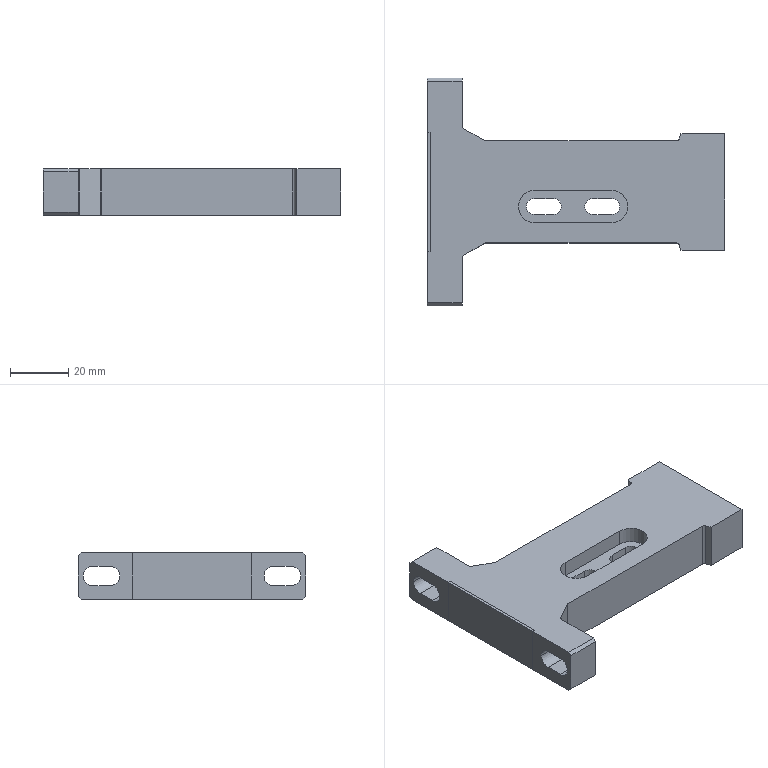NC program | NX | posted with a generic post | part box 102 x 78 x 16 mm
Lines 2750 to 3711 of 11044:
(ZLEVEL_PROFILE_COPY_COPY_1_COPY , TOOL : D4)
N5474 T04 M6
N5476 G54
N5478 G17 G0 G90 X-36. Y25.848 B0. C0. S9500 M3
N5480 G43 Z30. H4
N5482 Z-0.4
N5484 G94 G1 X-36.8 Y25.386 F1400.
N5486 G3 X-37. Y25.039 R0.4
N5488 G1 Y23.155
N5490 X-35.367 Y22.212
N5492 G3 X-34.967 Y22.212 R0.4
N5494 G1 X-34.167 Y22.674
N5496 G0 X-36. Y25.848 Z-0.8
N5498 G1 X-36.8 Y25.386
N5500 G3 X-37. Y25.039 R0.4
N5502 G1 Y23.155
N5504 X-35.367 Y22.212
N5506 G3 X-34.967 Y22.212 R0.4
N5508 G1 X-34.167 Y22.674
N5510 G0 X-36. Y25.848 Z-1.2
N5512 G1 X-36.8 Y25.386
N5514 G3 X-37. Y25.039 R0.4
N5516 G1 Y23.155
N5518 X-35.367 Y22.212
N5520 G3 X-34.967 Y22.212 R0.4
N5522 G1 X-34.167 Y22.674
N5524 G0 X-36. Y25.848 Z-1.6
N5526 G1 X-36.8 Y25.386
N5528 G3 X-37. Y25.039 R0.4
N5530 G1 Y23.155
N5532 X-35.367 Y22.212
N5534 G3 X-34.967 Y22.212 R0.4
N5536 G1 X-34.167 Y22.674
N5538 G0 X-36. Y25.848 Z-2.
N5540 G1 X-36.8 Y25.386
N5542 G3 X-37. Y25.039 R0.4
N5544 G1 Y23.155
N5546 X-35.367 Y22.212
N5548 G3 X-34.967 Y22.212 R0.4
N5550 G1 X-34.167 Y22.674
N5552 G0 X-36. Y25.848 Z-2.4
N5554 G1 X-36.8 Y25.386
N5556 G3 X-37. Y25.039 R0.4
N5558 G1 Y23.155
N5560 X-35.367 Y22.212
N5562 G3 X-34.967 Y22.212 R0.4
N5564 G1 X-34.167 Y22.674
N5566 G0 X-36. Y25.848 Z-2.8
N5568 G1 X-36.8 Y25.386
N5570 G3 X-37. Y25.039 R0.4
N5572 G1 Y23.155
N5574 X-35.367 Y22.212
N5576 G3 X-34.967 Y22.212 R0.4
N5578 G1 X-34.167 Y22.674
N5580 G0 X-36. Y25.848 Z-3.2
N5582 G1 X-36.8 Y25.386
N5584 G3 X-37. Y25.039 R0.4
N5586 G1 Y23.155
N5588 X-35.367 Y22.212
N5590 G3 X-34.967 Y22.212 R0.4
N5592 G1 X-34.167 Y22.674
N5594 G0 X-36. Y25.848 Z-3.6
N5596 G1 X-36.8 Y25.386
N5598 G3 X-37. Y25.039 R0.4
N5600 G1 Y23.155
N5602 X-35.367 Y22.212
N5604 G3 X-34.967 Y22.212 R0.4
N5606 G1 X-34.167 Y22.674
N5608 G0 X-36. Y25.848 Z-4.
N5610 G1 X-36.8 Y25.386
N5612 G3 X-37. Y25.039 R0.4
N5614 G1 Y23.155
N5616 X-35.367 Y22.212
N5618 G3 X-34.967 Y22.212 R0.4
N5620 G1 X-34.167 Y22.674
N5622 G0 X-36. Y25.848 Z-4.4
N5624 G1 X-36.8 Y25.386
N5626 G3 X-37. Y25.039 R0.4
N5628 G1 Y23.155
N5630 X-35.367 Y22.212
N5632 G3 X-34.967 Y22.212 R0.4
N5634 G1 X-34.167 Y22.674
N5636 G0 X-36. Y25.848 Z-4.8
N5638 G1 X-36.8 Y25.386
N5640 G3 X-37. Y25.039 R0.4
N5642 G1 Y23.155
N5644 X-35.367 Y22.212
N5646 G3 X-34.967 Y22.212 R0.4
N5648 G1 X-34.167 Y22.674
N5650 G0 X-36. Y25.848 Z-5.2
N5652 G1 X-36.8 Y25.386
N5654 G3 X-37. Y25.039 R0.4
N5656 G1 Y23.155
N5658 X-35.367 Y22.212
N5660 G3 X-34.967 Y22.212 R0.4
N5662 G1 X-34.167 Y22.674
N5664 G0 X-36. Y25.848 Z-5.6
N5666 G1 X-36.8 Y25.386
N5668 G3 X-37. Y25.039 R0.4
N5670 G1 Y23.155
N5672 X-35.367 Y22.212
N5674 G3 X-34.967 Y22.212 R0.4
N5676 G1 X-34.167 Y22.674
N5678 G0 X-36. Y25.848 Z-6.
N5680 G1 X-36.8 Y25.386
N5682 G3 X-37. Y25.039 R0.4
N5684 G1 Y23.155
N5686 X-35.367 Y22.212
N5688 G3 X-34.967 Y22.212 R0.4
N5690 G1 X-34.167 Y22.674
N5692 G0 X-36. Y25.848 Z-6.4
N5694 G1 X-36.8 Y25.386
N5696 G3 X-37. Y25.039 R0.4
N5698 G1 Y23.155
N5700 X-35.367 Y22.212
N5702 G3 X-34.967 Y22.212 R0.4
N5704 G1 X-34.167 Y22.674
N5706 G0 X-36. Y25.848 Z-6.8
N5708 G1 X-36.8 Y25.386
N5710 G3 X-37. Y25.039 R0.4
N5712 G1 Y23.155
N5714 X-35.367 Y22.212
N5716 G3 X-34.967 Y22.212 R0.4
N5718 G1 X-34.167 Y22.674
N5720 G0 X-36. Y25.848 Z-7.2
N5722 G1 X-36.8 Y25.386
N5724 G3 X-37. Y25.039 R0.4
N5726 G1 Y23.155
N5728 X-35.367 Y22.212
N5730 G3 X-34.967 Y22.212 R0.4
N5732 G1 X-34.167 Y22.674
N5734 G0 X-36. Y25.848 Z-7.6
N5736 G1 X-36.8 Y25.386
N5738 G3 X-37. Y25.039 R0.4
N5740 G1 Y23.155
N5742 X-35.367 Y22.212
N5744 G3 X-34.967 Y22.212 R0.4
N5746 G1 X-34.167 Y22.674
N5748 G0 X-36. Y25.848 Z-8.
N5750 G1 X-36.8 Y25.386
N5752 G3 X-37. Y25.039 R0.4
N5754 G1 Y23.155
N5756 X-35.367 Y22.212
N5758 G3 X-34.967 Y22.212 R0.4
N5760 G1 X-34.167 Y22.674
N5762 G0 X-36. Y25.848 Z-8.4
N5764 G1 X-36.8 Y25.386
N5766 G3 X-37. Y25.039 R0.4
N5768 G1 Y23.155
N5770 X-35.367 Y22.212
N5772 G3 X-34.967 Y22.212 R0.4
N5774 G1 X-34.167 Y22.674
N5776 G0 X-36. Y25.848 Z-8.8
N5778 G1 X-36.8 Y25.386
N5780 G3 X-37. Y25.039 R0.4
N5782 G1 Y23.155
N5784 X-35.367 Y22.212
N5786 G3 X-34.967 Y22.212 R0.4
N5788 G1 X-34.167 Y22.674
N5790 G0 X-36. Y25.848 Z-9.2
N5792 G1 X-36.8 Y25.386
N5794 G3 X-37. Y25.039 R0.4
N5796 G1 Y23.155
N5798 X-35.367 Y22.212
N5800 G3 X-34.967 Y22.212 R0.4
N5802 G1 X-34.167 Y22.674
N5804 G0 X-36. Y25.848 Z-9.6
N5806 G1 X-36.8 Y25.386
N5808 G3 X-37. Y25.039 R0.4
N5810 G1 Y23.155
N5812 X-35.367 Y22.212
N5814 G3 X-34.967 Y22.212 R0.4
N5816 G1 X-34.167 Y22.674
N5818 G0 X-36. Y25.848 Z-10.
N5820 G1 X-36.8 Y25.386
N5822 G3 X-37. Y25.039 R0.4
N5824 G1 Y23.155
N5826 X-35.367 Y22.212
N5828 G3 X-34.967 Y22.212 R0.4
N5830 G1 X-34.167 Y22.674
N5832 G0 X-36. Y25.848 Z-10.4
N5834 G1 X-36.8 Y25.386
N5836 G3 X-37. Y25.039 R0.4
N5838 G1 Y23.155
N5840 X-35.367 Y22.212
N5842 G3 X-34.967 Y22.212 R0.4
N5844 G1 X-34.167 Y22.674
N5846 G0 X-36. Y25.848 Z-10.8
N5848 G1 X-36.8 Y25.386
N5850 G3 X-37. Y25.039 R0.4
N5852 G1 Y23.155
N5854 X-35.367 Y22.212
N5856 G3 X-34.967 Y22.212 R0.4
N5858 G1 X-34.167 Y22.674
N5860 G0 X-36. Y25.848 Z-11.2
N5862 G1 X-36.8 Y25.386
N5864 G3 X-37. Y25.039 R0.4
N5866 G1 Y23.155
N5868 X-35.367 Y22.212
N5870 G3 X-34.967 Y22.212 R0.4
N5872 G1 X-34.167 Y22.674
N5874 G0 X-36. Y25.848 Z-11.6
N5876 G1 X-36.8 Y25.386
N5878 G3 X-37. Y25.039 R0.4
N5880 G1 Y23.155
N5882 X-35.367 Y22.212
N5884 G3 X-34.967 Y22.212 R0.4
N5886 G1 X-34.167 Y22.674
N5888 G0 X-36. Y25.848 Z-12.
N5890 G1 X-36.8 Y25.386
N5892 G3 X-37. Y25.039 R0.4
N5894 G1 Y23.155
N5896 X-35.367 Y22.212
N5898 G3 X-34.967 Y22.212 R0.4
N5900 G1 X-34.167 Y22.674
N5902 G0 X-36. Y25.848 Z-12.4
N5904 G1 X-36.8 Y25.386
N5906 G3 X-37. Y25.039 R0.4
N5908 G1 Y23.155
N5910 X-35.367 Y22.212
N5912 G3 X-34.967 Y22.212 R0.4
N5914 G1 X-34.167 Y22.674
N5916 G0 X-36. Y25.848 Z-12.8
N5918 G1 X-36.8 Y25.386
N5920 G3 X-37. Y25.039 R0.4
N5922 G1 Y23.155
N5924 X-35.367 Y22.212
N5926 G3 X-34.967 Y22.212 R0.4
N5928 G1 X-34.167 Y22.674
N5930 G0 X-36. Y25.848 Z-13.2
N5932 G1 X-36.8 Y25.386
N5934 G3 X-37. Y25.039 R0.4
N5936 G1 Y23.155
N5938 X-35.367 Y22.212
N5940 G3 X-34.967 Y22.212 R0.4
N5942 G1 X-34.167 Y22.674
N5944 G0 X-36. Y25.848 Z-13.6
N5946 G1 X-36.8 Y25.386
N5948 G3 X-37. Y25.039 R0.4
N5950 G1 Y23.155
N5952 X-35.367 Y22.212
N5954 G3 X-34.967 Y22.212 R0.4
N5956 G1 X-34.167 Y22.674
N5958 G0 X-36. Y25.848 Z-14.
N5960 G1 X-36.8 Y25.386
N5962 G3 X-37. Y25.039 R0.4
N5964 G1 Y23.155
N5966 X-35.367 Y22.212
N5968 G3 X-34.967 Y22.212 R0.4
N5970 G1 X-34.167 Y22.674
N5972 G0 X-36. Y25.848 Z-14.4
N5974 G1 X-36.8 Y25.386
N5976 G3 X-37. Y25.039 R0.4
N5978 G1 Y23.155
N5980 X-35.367 Y22.212
N5982 G3 X-34.967 Y22.212 R0.4
N5984 G1 X-34.167 Y22.674
N5986 G0 X-36. Y25.848 Z-14.8
N5988 G1 X-36.8 Y25.386
N5990 G3 X-37. Y25.039 R0.4
N5992 G1 Y23.155
N5994 X-35.367 Y22.212
N5996 G3 X-34.967 Y22.212 R0.4
N5998 G1 X-34.167 Y22.674
N6000 G0 X-36. Y25.848 Z-15.2
N6002 G1 X-36.8 Y25.386
N6004 G3 X-37. Y25.039 R0.4
N6006 G1 Y23.155
N6008 X-35.367 Y22.212
N6010 G3 X-34.967 Y22.212 R0.4
N6012 G1 X-34.167 Y22.674
N6014 G0 X-36. Y25.848 Z-15.6
N6016 G1 X-36.8 Y25.386
N6018 G3 X-37. Y25.039 R0.4
N6020 G1 Y23.155
N6022 X-35.367 Y22.212
N6024 G3 X-34.967 Y22.212 R0.4
N6026 G1 X-34.167 Y22.674
N6028 G0 X-36. Y25.848 Z-16.
N6030 G1 X-36.8 Y25.386
N6032 G3 X-37. Y25.039 R0.4
N6034 G1 Y23.155
N6036 X-35.367 Y22.212
N6038 G3 X-34.967 Y22.212 R0.4
N6040 G1 X-34.167 Y22.674
N6042 G0 Z30.
N6044 X-31.699 Y21.249
N6046 Z-0.4
N6048 G1 Y20.325
N6050 G3 X-31.499 Y19.978 R0.4
N6052 G1 X-30.67 Y19.5
N6054 X-29.713
N6056 G3 X-29.367 Y19.7 R0.4
N6058 G1 X-28.905 Y20.5
N6060 G0 X-31.699 Y21.249 Z-0.8
N6062 G1 Y20.325
N6064 G3 X-31.499 Y19.978 R0.4
N6066 G1 X-30.67 Y19.5
N6068 X-29.713
N6070 G3 X-29.367 Y19.7 R0.4
N6072 G1 X-28.905 Y20.5
N6074 G0 X-31.699 Y21.249 Z-1.2
N6076 G1 Y20.325
N6078 G3 X-31.499 Y19.978 R0.4
N6080 G1 X-30.67 Y19.5
N6082 X-29.713
N6084 G3 X-29.367 Y19.7 R0.4
N6086 G1 X-28.905 Y20.5
N6088 G0 X-31.699 Y21.249 Z-1.6
N6090 G1 Y20.325
N6092 G3 X-31.499 Y19.978 R0.4
N6094 G1 X-30.67 Y19.5
N6096 X-29.713
N6098 G3 X-29.367 Y19.7 R0.4
N6100 G1 X-28.905 Y20.5
N6102 G0 X-31.699 Y21.249 Z-2.
N6104 G1 Y20.325
N6106 G3 X-31.499 Y19.978 R0.4
N6108 G1 X-30.67 Y19.5
N6110 X-29.713
N6112 G3 X-29.367 Y19.7 R0.4
N6114 G1 X-28.905 Y20.5
N6116 G0 X-31.699 Y21.249 Z-2.4
N6118 G1 Y20.325
N6120 G3 X-31.499 Y19.978 R0.4
N6122 G1 X-30.67 Y19.5
N6124 X-29.713
N6126 G3 X-29.367 Y19.7 R0.4
N6128 G1 X-28.905 Y20.5
N6130 G0 X-31.699 Y21.249 Z-2.8
N6132 G1 Y20.325
N6134 G3 X-31.499 Y19.978 R0.4
N6136 G1 X-30.67 Y19.5
N6138 X-29.713
N6140 G3 X-29.367 Y19.7 R0.4
N6142 G1 X-28.905 Y20.5
N6144 G0 X-31.699 Y21.249 Z-3.2
N6146 G1 Y20.325
N6148 G3 X-31.499 Y19.978 R0.4
N6150 G1 X-30.67 Y19.5
N6152 X-29.713
N6154 G3 X-29.367 Y19.7 R0.4
N6156 G1 X-28.905 Y20.5
N6158 G0 X-31.699 Y21.249 Z-3.6
N6160 G1 Y20.325
N6162 G3 X-31.499 Y19.978 R0.4
N6164 G1 X-30.67 Y19.5
N6166 X-29.713
N6168 G3 X-29.367 Y19.7 R0.4
N6170 G1 X-28.905 Y20.5
N6172 G0 X-31.699 Y21.249 Z-4.
N6174 G1 Y20.325
N6176 G3 X-31.499 Y19.978 R0.4
N6178 G1 X-30.67 Y19.5
N6180 X-29.713
N6182 G3 X-29.367 Y19.7 R0.4
N6184 G1 X-28.905 Y20.5
N6186 G0 X-31.699 Y21.249 Z-4.4
N6188 G1 Y20.325
N6190 G3 X-31.499 Y19.978 R0.4
N6192 G1 X-30.67 Y19.5
N6194 X-29.713
N6196 G3 X-29.367 Y19.7 R0.4
N6198 G1 X-28.905 Y20.5
N6200 G0 X-31.699 Y21.249 Z-4.8
N6202 G1 Y20.325
N6204 G3 X-31.499 Y19.978 R0.4
N6206 G1 X-30.67 Y19.5
N6208 X-29.713
N6210 G3 X-29.367 Y19.7 R0.4
N6212 G1 X-28.905 Y20.5
N6214 G0 X-31.699 Y21.249 Z-5.2
N6216 G1 Y20.325
N6218 G3 X-31.499 Y19.978 R0.4
N6220 G1 X-30.67 Y19.5
N6222 X-29.713
N6224 G3 X-29.367 Y19.7 R0.4
N6226 G1 X-28.905 Y20.5
N6228 G0 X-31.699 Y21.249 Z-5.6
N6230 G1 Y20.325
N6232 G3 X-31.499 Y19.978 R0.4
N6234 G1 X-30.67 Y19.5
N6236 X-29.713
N6238 G3 X-29.367 Y19.7 R0.4
N6240 G1 X-28.905 Y20.5
N6242 G0 X-31.699 Y21.249 Z-6.
N6244 G1 Y20.325
N6246 G3 X-31.499 Y19.978 R0.4
N6248 G1 X-30.67 Y19.5
N6250 X-29.713
N6252 G3 X-29.367 Y19.7 R0.4
N6254 G1 X-28.905 Y20.5
N6256 G0 X-31.699 Y21.249 Z-6.4
N6258 G1 Y20.325
N6260 G3 X-31.499 Y19.978 R0.4
N6262 G1 X-30.67 Y19.5
N6264 X-29.713
N6266 G3 X-29.367 Y19.7 R0.4
N6268 G1 X-28.905 Y20.5
N6270 G0 X-31.699 Y21.249 Z-6.8
N6272 G1 Y20.325
N6274 G3 X-31.499 Y19.978 R0.4
N6276 G1 X-30.67 Y19.5
N6278 X-29.713
N6280 G3 X-29.367 Y19.7 R0.4
N6282 G1 X-28.905 Y20.5
N6284 G0 X-31.699 Y21.249 Z-7.2
N6286 G1 Y20.325
N6288 G3 X-31.499 Y19.978 R0.4
N6290 G1 X-30.67 Y19.5
N6292 X-29.713
N6294 G3 X-29.367 Y19.7 R0.4
N6296 G1 X-28.905 Y20.5
N6298 G0 X-31.699 Y21.249 Z-7.6
N6300 G1 Y20.325
N6302 G3 X-31.499 Y19.978 R0.4
N6304 G1 X-30.67 Y19.5
N6306 X-29.713
N6308 G3 X-29.367 Y19.7 R0.4
N6310 G1 X-28.905 Y20.5
N6312 G0 X-31.699 Y21.249 Z-8.
N6314 G1 Y20.325
N6316 G3 X-31.499 Y19.978 R0.4
N6318 G1 X-30.67 Y19.5
N6320 X-29.713
N6322 G3 X-29.367 Y19.7 R0.4
N6324 G1 X-28.905 Y20.5
N6326 G0 X-31.699 Y21.249 Z-8.4
N6328 G1 Y20.325
N6330 G3 X-31.499 Y19.978 R0.4
N6332 G1 X-30.67 Y19.5
N6334 X-29.713
N6336 G3 X-29.367 Y19.7 R0.4
N6338 G1 X-28.905 Y20.5
N6340 G0 X-31.699 Y21.249 Z-8.8
N6342 G1 Y20.325
N6344 G3 X-31.499 Y19.978 R0.4
N6346 G1 X-30.67 Y19.5
N6348 X-29.713
N6350 G3 X-29.367 Y19.7 R0.4
N6352 G1 X-28.905 Y20.5
N6354 G0 X-31.699 Y21.249 Z-9.2
N6356 G1 Y20.325
N6358 G3 X-31.499 Y19.978 R0.4
N6360 G1 X-30.67 Y19.5
N6362 X-29.713
N6364 G3 X-29.367 Y19.7 R0.4
N6366 G1 X-28.905 Y20.5
N6368 G0 X-31.699 Y21.249 Z-9.6
N6370 G1 Y20.325
N6372 G3 X-31.499 Y19.978 R0.4
N6374 G1 X-30.67 Y19.5
N6376 X-29.713
N6378 G3 X-29.367 Y19.7 R0.4
N6380 G1 X-28.905 Y20.5
N6382 G0 X-31.699 Y21.249 Z-10.
N6384 G1 Y20.325
N6386 G3 X-31.499 Y19.978 R0.4
N6388 G1 X-30.67 Y19.5
N6390 X-29.713
N6392 G3 X-29.367 Y19.7 R0.4
N6394 G1 X-28.905 Y20.5
N6396 G0 X-31.699 Y21.249 Z-10.4
N6398 G1 Y20.325
N6400 G3 X-31.499 Y19.978 R0.4
N6402 G1 X-30.67 Y19.5
N6404 X-29.713
N6406 G3 X-29.367 Y19.7 R0.4
N6408 G1 X-28.905 Y20.5
N6410 G0 X-31.699 Y21.249 Z-10.8
N6412 G1 Y20.325
N6414 G3 X-31.499 Y19.978 R0.4
N6416 G1 X-30.67 Y19.5
N6418 X-29.713
N6420 G3 X-29.367 Y19.7 R0.4
N6422 G1 X-28.905 Y20.5
N6424 G0 X-31.699 Y21.249 Z-11.2
N6426 G1 Y20.325
N6428 G3 X-31.499 Y19.978 R0.4
N6430 G1 X-30.67 Y19.5
N6432 X-29.713
N6434 G3 X-29.367 Y19.7 R0.4
N6436 G1 X-28.905 Y20.5
N6438 G0 X-31.699 Y21.249 Z-11.6
N6440 G1 Y20.325
N6442 G3 X-31.499 Y19.978 R0.4
N6444 G1 X-30.67 Y19.5
N6446 X-29.713
N6448 G3 X-29.367 Y19.7 R0.4
N6450 G1 X-28.905 Y20.5
N6452 G0 X-31.699 Y21.249 Z-12.
N6454 G1 Y20.325
N6456 G3 X-31.499 Y19.978 R0.4
N6458 G1 X-30.67 Y19.5
N6460 X-29.713
N6462 G3 X-29.367 Y19.7 R0.4
N6464 G1 X-28.905 Y20.5
N6466 G0 X-31.699 Y21.249 Z-12.4
N6468 G1 Y20.325
N6470 G3 X-31.499 Y19.978 R0.4
N6472 G1 X-30.67 Y19.5
N6474 X-29.713
N6476 G3 X-29.367 Y19.7 R0.4
N6478 G1 X-28.905 Y20.5
N6480 G0 X-31.699 Y21.249 Z-12.8
N6482 G1 Y20.325
N6484 G3 X-31.499 Y19.978 R0.4
N6486 G1 X-30.67 Y19.5
N6488 X-29.713
N6490 G3 X-29.367 Y19.7 R0.4
N6492 G1 X-28.905 Y20.5
N6494 G0 X-31.699 Y21.249 Z-13.2
N6496 G1 Y20.325
N6498 G3 X-31.499 Y19.978 R0.4
N6500 G1 X-30.67 Y19.5
N6502 X-29.713
N6504 G3 X-29.367 Y19.7 R0.4
N6506 G1 X-28.905 Y20.5
N6508 G0 X-31.699 Y21.249 Z-13.6
N6510 G1 Y20.325
N6512 G3 X-31.499 Y19.978 R0.4
N6514 G1 X-30.67 Y19.5
N6516 X-29.713
N6518 G3 X-29.367 Y19.7 R0.4
N6520 G1 X-28.905 Y20.5
N6522 G0 X-31.699 Y21.249 Z-14.
N6524 G1 Y20.325
N6526 G3 X-31.499 Y19.978 R0.4
N6528 G1 X-30.67 Y19.5
N6530 X-29.713
N6532 G3 X-29.367 Y19.7 R0.4
N6534 G1 X-28.905 Y20.5
N6536 G0 X-31.699 Y21.249 Z-14.4
N6538 G1 Y20.325
N6540 G3 X-31.499 Y19.978 R0.4
N6542 G1 X-30.67 Y19.5
N6544 X-29.713
N6546 G3 X-29.367 Y19.7 R0.4
N6548 G1 X-28.905 Y20.5
N6550 G0 X-31.699 Y21.249 Z-14.8
N6552 G1 Y20.325
N6554 G3 X-31.499 Y19.978 R0.4
N6556 G1 X-30.67 Y19.5
N6558 X-29.713
N6560 G3 X-29.367 Y19.7 R0.4
N6562 G1 X-28.905 Y20.5
N6564 G0 X-31.699 Y21.249 Z-15.2
N6566 G1 Y20.325
N6568 G3 X-31.499 Y19.978 R0.4
N6570 G1 X-30.67 Y19.5
N6572 X-29.713
N6574 G3 X-29.367 Y19.7 R0.4
N6576 G1 X-28.905 Y20.5
N6578 G0 X-31.699 Y21.249 Z-15.6
N6580 G1 Y20.325
N6582 G3 X-31.499 Y19.978 R0.4
N6584 G1 X-30.67 Y19.5
N6586 X-29.713
N6588 G3 X-29.367 Y19.7 R0.4
N6590 G1 X-28.905 Y20.5
N6592 G0 X-31.699 Y21.249 Z-16.
N6594 G1 Y20.325
N6596 G3 X-31.499 Y19.978 R0.4
N6598 G1 X-30.67 Y19.5
N6600 X-29.713
N6602 G3 X-29.367 Y19.7 R0.4
N6604 G1 X-28.905 Y20.5
N6606 G0 Z30.
N6608 X30.709
N6610 Z-0.4
N6612 G1 X31.17 Y19.7
N6614 G3 X31.517 Y19.5 R0.4
N6616 G1 X33.69
N6618 X34.121 Y20.684
N6620 G2 X34.426 Y21.233 R2.
N6622 G3 X34.482 Y21.629 R0.4
N6624 G1 X34.178 Y22.383
N6626 G0 X30.709 Y20.5 Z-0.8
N6628 G1 X31.17 Y19.7
N6630 G3 X31.517 Y19.5 R0.4
N6632 G1 X33.69
N6634 X34.121 Y20.684
N6636 G2 X34.426 Y21.233 R2.
N6638 G3 X34.482 Y21.629 R0.4
N6640 G1 X34.178 Y22.383
N6642 G0 X30.709 Y20.5 Z-1.2
N6644 G1 X31.17 Y19.7
N6646 G3 X31.517 Y19.5 R0.4
N6648 G1 X33.69
N6650 X34.121 Y20.684
N6652 G2 X34.426 Y21.233 R2.
N6654 G3 X34.482 Y21.629 R0.4
N6656 G1 X34.178 Y22.383
N6658 G0 X30.709 Y20.5 Z-1.6
N6660 G1 X31.17 Y19.7
N6662 G3 X31.517 Y19.5 R0.4
N6664 G1 X33.69
N6666 X34.121 Y20.684
N6668 G2 X34.426 Y21.233 R2.
N6670 G3 X34.482 Y21.629 R0.4
N6672 G1 X34.178 Y22.383
N6674 G0 X30.709 Y20.5 Z-2.
N6676 G1 X31.17 Y19.7
N6678 G3 X31.517 Y19.5 R0.4
N6680 G1 X33.69
N6682 X34.121 Y20.684
N6684 G2 X34.426 Y21.233 R2.
N6686 G3 X34.482 Y21.629 R0.4
N6688 G1 X34.178 Y22.383
N6690 G0 X30.709 Y20.5 Z-2.4
N6692 G1 X31.17 Y19.7
N6694 G3 X31.517 Y19.5 R0.4
N6696 G1 X33.69
N6698 X34.121 Y20.684
N6700 G2 X34.426 Y21.233 R2.
N6702 G3 X34.482 Y21.629 R0.4
N6704 G1 X34.178 Y22.383
N6706 G0 X30.709 Y20.5 Z-2.8
N6708 G1 X31.17 Y19.7
N6710 G3 X31.517 Y19.5 R0.4
N6712 G1 X33.69
N6714 X34.121 Y20.684
N6716 G2 X34.426 Y21.233 R2.
N6718 G3 X34.482 Y21.629 R0.4
N6720 G1 X34.178 Y22.383
N6722 G0 X30.709 Y20.5 Z-3.2
N6724 G1 X31.17 Y19.7
N6726 G3 X31.517 Y19.5 R0.4
N6728 G1 X33.69
N6730 X34.121 Y20.684
N6732 G2 X34.426 Y21.233 R2.
N6734 G3 X34.482 Y21.629 R0.4
N6736 G1 X34.178 Y22.383
N6738 G0 X30.709 Y20.5 Z-3.6
N6740 G1 X31.17 Y19.7
N6742 G3 X31.517 Y19.5 R0.4
N6744 G1 X33.69
N6746 X34.121 Y20.684
N6748 G2 X34.426 Y21.233 R2.
N6750 G3 X34.482 Y21.629 R0.4
N6752 G1 X34.178 Y22.383
N6754 G0 X30.709 Y20.5 Z-4.
N6756 G1 X31.17 Y19.7
N6758 G3 X31.517 Y19.5 R0.4
N6760 G1 X33.69
N6762 X34.121 Y20.684
N6764 G2 X34.426 Y21.233 R2.
N6766 G3 X34.482 Y21.629 R0.4
N6768 G1 X34.178 Y22.383
N6770 G0 X30.709 Y20.5 Z-4.4
N6772 G1 X31.17 Y19.7
N6774 G3 X31.517 Y19.5 R0.4
N6776 G1 X33.69
N6778 X34.121 Y20.684
N6780 G2 X34.426 Y21.233 R2.
N6782 G3 X34.482 Y21.629 R0.4
N6784 G1 X34.178 Y22.383
N6786 G0 X30.709 Y20.5 Z-4.8
N6788 G1 X31.17 Y19.7
N6790 G3 X31.517 Y19.5 R0.4
N6792 G1 X33.69
N6794 X34.121 Y20.684
N6796 G2 X34.426 Y21.233 R2.
N6798 G3 X34.482 Y21.629 R0.4
N6800 G1 X34.178 Y22.383
N6802 G0 X30.709 Y20.5 Z-5.2
N6804 G1 X31.17 Y19.7
N6806 G3 X31.517 Y19.5 R0.4
N6808 G1 X33.69
N6810 X34.121 Y20.684
N6812 G2 X34.426 Y21.233 R2.
N6814 G3 X34.482 Y21.629 R0.4
N6816 G1 X34.178 Y22.383
N6818 G0 X30.709 Y20.5 Z-5.6
N6820 G1 X31.17 Y19.7
N6822 G3 X31.517 Y19.5 R0.4
N6824 G1 X33.69
N6826 X34.121 Y20.684
N6828 G2 X34.426 Y21.233 R2.
N6830 G3 X34.482 Y21.629 R0.4
N6832 G1 X34.178 Y22.383
N6834 G0 X30.709 Y20.5 Z-6.
N6836 G1 X31.17 Y19.7
N6838 G3 X31.517 Y19.5 R0.4
N6840 G1 X33.69
N6842 X34.121 Y20.684
N6844 G2 X34.426 Y21.233 R2.
N6846 G3 X34.482 Y21.629 R0.4
N6848 G1 X34.178 Y22.383
N6850 G0 X30.709 Y20.5 Z-6.4
N6852 G1 X31.17 Y19.7
N6854 G3 X31.517 Y19.5 R0.4
N6856 G1 X33.69
N6858 X34.121 Y20.684
N6860 G2 X34.426 Y21.233 R2.
N6862 G3 X34.482 Y21.629 R0.4
N6864 G1 X34.178 Y22.383
N6866 G0 X30.709 Y20.5 Z-6.8
N6868 G1 X31.17 Y19.7
N6870 G3 X31.517 Y19.5 R0.4
N6872 G1 X33.69
N6874 X34.121 Y20.684
N6876 G2 X34.426 Y21.233 R2.
N6878 G3 X34.482 Y21.629 R0.4
N6880 G1 X34.178 Y22.383
N6882 G0 X30.709 Y20.5 Z-7.2
N6884 G1 X31.17 Y19.7
N6886 G3 X31.517 Y19.5 R0.4
N6888 G1 X33.69
N6890 X34.121 Y20.684
N6892 G2 X34.426 Y21.233 R2.
N6894 G3 X34.482 Y21.629 R0.4
N6896 G1 X34.178 Y22.383
N6898 G0 X30.709 Y20.5 Z-7.6
N6900 G1 X31.17 Y19.7
N6902 G3 X31.517 Y19.5 R0.4
N6904 G1 X33.69
N6906 X34.121 Y20.684
N6908 G2 X34.426 Y21.233 R2.
N6910 G3 X34.482 Y21.629 R0.4
N6912 G1 X34.178 Y22.383
N6914 G0 X30.709 Y20.5 Z-8.
N6916 G1 X31.17 Y19.7
N6918 G3 X31.517 Y19.5 R0.4
N6920 G1 X33.69
N6922 X34.121 Y20.684
N6924 G2 X34.426 Y21.233 R2.
N6926 G3 X34.482 Y21.629 R0.4
N6928 G1 X34.178 Y22.383
N6930 G0 X30.709 Y20.5 Z-8.4
N6932 G1 X31.17 Y19.7
N6934 G3 X31.517 Y19.5 R0.4
N6936 G1 X33.69
N6938 X34.121 Y20.684
N6940 G2 X34.426 Y21.233 R2.
N6942 G3 X34.482 Y21.629 R0.4
N6944 G1 X34.178 Y22.383
N6946 G0 X30.709 Y20.5 Z-8.8
N6948 G1 X31.17 Y19.7
N6950 G3 X31.517 Y19.5 R0.4
N6952 G1 X33.69
N6954 X34.121 Y20.684
N6956 G2 X34.426 Y21.233 R2.
N6958 G3 X34.482 Y21.629 R0.4
N6960 G1 X34.178 Y22.383
N6962 G0 X30.709 Y20.5 Z-9.2
N6964 G1 X31.17 Y19.7
N6966 G3 X31.517 Y19.5 R0.4
N6968 G1 X33.69
N6970 X34.121 Y20.684
N6972 G2 X34.426 Y21.233 R2.
N6974 G3 X34.482 Y21.629 R0.4
N6976 G1 X34.178 Y22.383
N6978 G0 X30.709 Y20.5 Z-9.6
N6980 G1 X31.17 Y19.7
N6982 G3 X31.517 Y19.5 R0.4
N6984 G1 X33.69
N6986 X34.121 Y20.684
N6988 G2 X34.426 Y21.233 R2.
N6990 G3 X34.482 Y21.629 R0.4
N6992 G1 X34.178 Y22.383
N6994 G0 X30.709 Y20.5 Z-10.
N6996 G1 X31.17 Y19.7
N6998 G3 X31.517 Y19.5 R0.4
N7000 G1 X33.69
N7002 X34.121 Y20.684
N7004 G2 X34.426 Y21.233 R2.
N7006 G3 X34.482 Y21.629 R0.4
N7008 G1 X34.178 Y22.383
N7010 G0 X30.709 Y20.5 Z-10.4
N7012 G1 X31.17 Y19.7
N7014 G3 X31.517 Y19.5 R0.4
N7016 G1 X33.69
N7018 X34.121 Y20.684
N7020 G2 X34.426 Y21.233 R2.
N7022 G3 X34.482 Y21.629 R0.4
N7024 G1 X34.178 Y22.383
N7026 G0 X30.709 Y20.5 Z-10.8
N7028 G1 X31.17 Y19.7
N7030 G3 X31.517 Y19.5 R0.4
N7032 G1 X33.69
N7034 X34.121 Y20.684
N7036 G2 X34.426 Y21.233 R2.
N7038 G3 X34.482 Y21.629 R0.4
N7040 G1 X34.178 Y22.383
N7042 G0 X30.709 Y20.5 Z-11.2
N7044 G1 X31.17 Y19.7
N7046 G3 X31.517 Y19.5 R0.4
N7048 G1 X33.69
N7050 X34.121 Y20.684
N7052 G2 X34.426 Y21.233 R2.
N7054 G3 X34.482 Y21.629 R0.4
N7056 G1 X34.178 Y22.383
N7058 G0 X30.709 Y20.5 Z-11.6
N7060 G1 X31.17 Y19.7
N7062 G3 X31.517 Y19.5 R0.4
N7064 G1 X33.69
N7066 X34.121 Y20.684
N7068 G2 X34.426 Y21.233 R2.
N7070 G3 X34.482 Y21.629 R0.4
N7072 G1 X34.178 Y22.383
N7074 G0 X30.709 Y20.5 Z-12.
N7076 G1 X31.17 Y19.7
N7078 G3 X31.517 Y19.5 R0.4
N7080 G1 X33.69
N7082 X34.121 Y20.684
N7084 G2 X34.426 Y21.233 R2.
N7086 G3 X34.482 Y21.629 R0.4
N7088 G1 X34.178 Y22.383
N7090 G0 X30.709 Y20.5 Z-12.4
N7092 G1 X31.17 Y19.7
N7094 G3 X31.517 Y19.5 R0.4
N7096 G1 X33.69
N7098 X34.121 Y20.684
N7100 G2 X34.426 Y21.233 R2.
N7102 G3 X34.482 Y21.629 R0.4
N7104 G1 X34.178 Y22.383
N7106 G0 X30.709 Y20.5 Z-12.8
N7108 G1 X31.17 Y19.7
N7110 G3 X31.517 Y19.5 R0.4
N7112 G1 X33.69
N7114 X34.121 Y20.684
N7116 G2 X34.426 Y21.233 R2.
N7118 G3 X34.482 Y21.629 R0.4
N7120 G1 X34.178 Y22.383
N7122 G0 X30.709 Y20.5 Z-13.2
N7124 G1 X31.17 Y19.7
N7126 G3 X31.517 Y19.5 R0.4
N7128 G1 X33.69
N7130 X34.121 Y20.684
N7132 G2 X34.426 Y21.233 R2.
N7134 G3 X34.482 Y21.629 R0.4
N7136 G1 X34.178 Y22.383
N7138 G0 X30.709 Y20.5 Z-13.6
N7140 G1 X31.17 Y19.7
N7142 G3 X31.517 Y19.5 R0.4
N7144 G1 X33.69
N7146 X34.121 Y20.684
N7148 G2 X34.426 Y21.233 R2.
N7150 G3 X34.482 Y21.629 R0.4
N7152 G1 X34.178 Y22.383
N7154 G0 X30.709 Y20.5 Z-14.
N7156 G1 X31.17 Y19.7
N7158 G3 X31.517 Y19.5 R0.4
N7160 G1 X33.69
N7162 X34.121 Y20.684
N7164 G2 X34.426 Y21.233 R2.
N7166 G3 X34.482 Y21.629 R0.4
N7168 G1 X34.178 Y22.383
N7170 G0 X30.709 Y20.5 Z-14.4
N7172 G1 X31.17 Y19.7
N7174 G3 X31.517 Y19.5 R0.4
N7176 G1 X33.69
N7178 X34.121 Y20.684
N7180 G2 X34.426 Y21.233 R2.
N7182 G3 X34.482 Y21.629 R0.4
N7184 G1 X34.178 Y22.383
N7186 G0 X30.709 Y20.5 Z-14.8
N7188 G1 X31.17 Y19.7
N7190 G3 X31.517 Y19.5 R0.4
N7192 G1 X33.69
N7194 X34.121 Y20.684
N7196 G2 X34.426 Y21.233 R2.
N7198 G3 X34.482 Y21.629 R0.4
N7200 G1 X34.178 Y22.383
N7202 G0 X30.709 Y20.5 Z-15.2
N7204 G1 X31.17 Y19.7
N7206 G3 X31.517 Y19.5 R0.4
N7208 G1 X33.69
N7210 X34.121 Y20.684
N7212 G2 X34.426 Y21.233 R2.
N7214 G3 X34.482 Y21.629 R0.4
N7216 G1 X34.178 Y22.383
N7218 G0 X30.709 Y20.5 Z-15.6
N7220 G1 X31.17 Y19.7
N7222 G3 X31.517 Y19.5 R0.4
N7224 G1 X33.69
N7226 X34.121 Y20.684
N7228 G2 X34.426 Y21.233 R2.
N7230 G3 X34.482 Y21.629 R0.4
N7232 G1 X34.178 Y22.383
N7234 G0 X30.709 Y20.5 Z-16.
N7236 G1 X31.17 Y19.7
N7238 G3 X31.517 Y19.5 R0.4
N7240 G1 X33.69
N7242 X34.121 Y20.684
N7244 G2 X34.426 Y21.233 R2.
N7246 G3 X34.482 Y21.629 R0.4
N7248 G1 X34.178 Y22.383
N7250 G0 Z30.
N7252 Y-22.383
N7254 Z-0.4
N7256 G1 X34.482 Y-21.629
N7258 G3 X34.426 Y-21.233 R0.4
N7260 G2 X34.121 Y-20.684 R2.
N7262 G1 X33.69 Y-19.5
N7264 X31.517
N7266 G3 X31.17 Y-19.7 R0.4
N7268 G1 X30.709 Y-20.5
N7270 G0 X34.178 Y-22.383 Z-0.8
N7272 G1 X34.482 Y-21.629
N7274 G3 X34.426 Y-21.233 R0.4
N7276 G2 X34.121 Y-20.684 R2.
N7278 G1 X33.69 Y-19.5
N7280 X31.517
N7282 G3 X31.17 Y-19.7 R0.4
N7284 G1 X30.709 Y-20.5
N7286 G0 X34.178 Y-22.383 Z-1.2
N7288 G1 X34.482 Y-21.629
N7290 G3 X34.426 Y-21.233 R0.4
N7292 G2 X34.121 Y-20.684 R2.
N7294 G1 X33.69 Y-19.5
N7296 X31.517
N7298 G3 X31.17 Y-19.7 R0.4
N7300 G1 X30.709 Y-20.5
N7302 G0 X34.178 Y-22.383 Z-1.6
N7304 G1 X34.482 Y-21.629
N7306 G3 X34.426 Y-21.233 R0.4
N7308 G2 X34.121 Y-20.684 R2.
N7310 G1 X33.69 Y-19.5
N7312 X31.517
N7314 G3 X31.17 Y-19.7 R0.4
N7316 G1 X30.709 Y-20.5
N7318 G0 X34.178 Y-22.383 Z-2.
N7320 G1 X34.482 Y-21.629
N7322 G3 X34.426 Y-21.233 R0.4
N7324 G2 X34.121 Y-20.684 R2.
N7326 G1 X33.69 Y-19.5
N7328 X31.517
N7330 G3 X31.17 Y-19.7 R0.4
N7332 G1 X30.709 Y-20.5
N7334 G0 X34.178 Y-22.383 Z-2.4
N7336 G1 X34.482 Y-21.629
N7338 G3 X34.426 Y-21.233 R0.4
N7340 G2 X34.121 Y-20.684 R2.
N7342 G1 X33.69 Y-19.5
N7344 X31.517
N7346 G3 X31.17 Y-19.7 R0.4
N7348 G1 X30.709 Y-20.5
N7350 G0 X34.178 Y-22.383 Z-2.8
N7352 G1 X34.482 Y-21.629
N7354 G3 X34.426 Y-21.233 R0.4
N7356 G2 X34.121 Y-20.684 R2.
N7358 G1 X33.69 Y-19.5
N7360 X31.517
N7362 G3 X31.17 Y-19.7 R0.4
N7364 G1 X30.709 Y-20.5
N7366 G0 X34.178 Y-22.383 Z-3.2
N7368 G1 X34.482 Y-21.629
N7370 G3 X34.426 Y-21.233 R0.4
N7372 G2 X34.121 Y-20.684 R2.
N7374 G1 X33.69 Y-19.5
N7376 X31.517
N7378 G3 X31.17 Y-19.7 R0.4
N7380 G1 X30.709 Y-20.5
N7382 G0 X34.178 Y-22.383 Z-3.6
N7384 G1 X34.482 Y-21.629
N7386 G3 X34.426 Y-21.233 R0.4
N7388 G2 X34.121 Y-20.684 R2.
N7390 G1 X33.69 Y-19.5